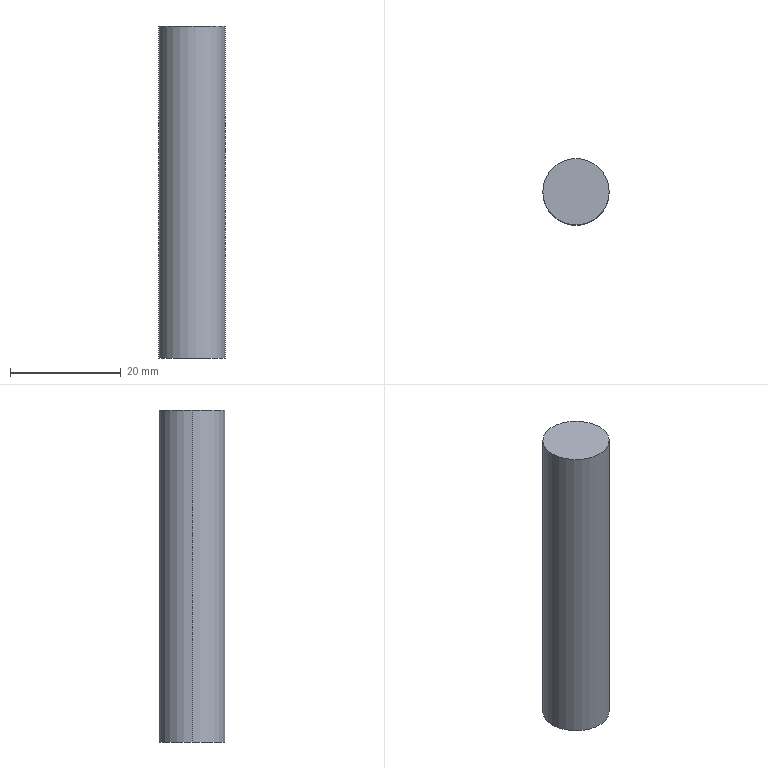Part | SolidWorks | features Extrusion 1 | 1 solid | 4 faces | box 12 x 12 x 60 mm | volume 6786 mm3 | cylinder 2 | plane 2 | commonest cylinder face diameters 12 x2
STEP:
#1=CARTESIAN_POINT('',(6.,0.,-30.));
#2=VERTEX_POINT('',#1);
#3=CARTESIAN_POINT('',(-6.,0.,-30.));
#4=VERTEX_POINT('',#3);
#5=CARTESIAN_POINT('',(0.,0.,-30.));
#6=DIRECTION('',(0.,0.,1.));
#7=DIRECTION('',(1.,0.,0.));
#8=AXIS2_PLACEMENT_3D('',#5,#6,#7);
#9=CIRCLE('',#8,6.);
#10=EDGE_CURVE('',#2,#4,#9,.T.);
#11=ORIENTED_EDGE('',*,*,#10,.T.);
#12=CARTESIAN_POINT('',(-6.,0.,30.));
#13=VERTEX_POINT('',#12);
#14=CARTESIAN_POINT('',(-6.,0.,-30.));
#15=DIRECTION('',(0.,0.,1.));
#16=VECTOR('',#15,1000.);
#17=LINE('',#14,#16);
#18=EDGE_CURVE('',#4,#13,#17,.T.);
#19=ORIENTED_EDGE('',*,*,#18,.T.);
#20=CARTESIAN_POINT('',(6.,0.,30.));
#21=VERTEX_POINT('',#20);
#22=CARTESIAN_POINT('',(0.,0.,30.));
#23=DIRECTION('',(0.,0.,1.));
#24=DIRECTION('',(1.,0.,0.));
#25=AXIS2_PLACEMENT_3D('',#22,#23,#24);
#26=CIRCLE('',#25,6.);
#27=EDGE_CURVE('',#21,#13,#26,.T.);
#28=ORIENTED_EDGE('',*,*,#27,.F.);
#29=CARTESIAN_POINT('',(6.,0.,-30.));
#30=DIRECTION('',(0.,0.,1.));
#31=VECTOR('',#30,1000.);
#32=LINE('',#29,#31);
#33=EDGE_CURVE('',#2,#21,#32,.T.);
#34=ORIENTED_EDGE('',*,*,#33,.F.);
#35=EDGE_LOOP('',(#11,#19,#28,#34));
#36=FACE_OUTER_BOUND('',#35,.T.);
#37=CARTESIAN_POINT('',(0.,0.,-30.));
#38=DIRECTION('',(0.,0.,1.));
#39=DIRECTION('',(1.,0.,0.));
#40=AXIS2_PLACEMENT_3D('',#37,#38,#39);
#41=CYLINDRICAL_SURFACE('',#40,6.);
#42=ADVANCED_FACE('',(#36),#41,.T.);
#43=ORIENTED_EDGE('',*,*,#18,.F.);
#44=CARTESIAN_POINT('',(0.,0.,-30.));
#45=DIRECTION('',(0.,0.,1.));
#46=DIRECTION('',(1.,0.,0.));
#47=AXIS2_PLACEMENT_3D('',#44,#45,#46);
#48=CIRCLE('',#47,6.);
#49=EDGE_CURVE('',#4,#2,#48,.T.);
#50=ORIENTED_EDGE('',*,*,#49,.T.);
#51=ORIENTED_EDGE('',*,*,#33,.T.);
#52=CARTESIAN_POINT('',(0.,0.,30.));
#53=DIRECTION('',(0.,0.,1.));
#54=DIRECTION('',(1.,0.,0.));
#55=AXIS2_PLACEMENT_3D('',#52,#53,#54);
#56=CIRCLE('',#55,6.);
#57=EDGE_CURVE('',#13,#21,#56,.T.);
#58=ORIENTED_EDGE('',*,*,#57,.F.);
#59=EDGE_LOOP('',(#43,#50,#51,#58));
#60=FACE_OUTER_BOUND('',#59,.T.);
#61=CARTESIAN_POINT('',(0.,0.,-30.));
#62=DIRECTION('',(0.,0.,1.));
#63=DIRECTION('',(1.,0.,0.));
#64=AXIS2_PLACEMENT_3D('',#61,#62,#63);
#65=CYLINDRICAL_SURFACE('',#64,6.);
#66=ADVANCED_FACE('',(#60),#65,.T.);
#67=ORIENTED_EDGE('',*,*,#10,.F.);
#68=ORIENTED_EDGE('',*,*,#49,.F.);
#69=EDGE_LOOP('',(#67,#68));
#70=FACE_OUTER_BOUND('',#69,.T.);
#71=CARTESIAN_POINT('',(0.,0.,-30.));
#72=DIRECTION('',(0.,0.,1.));
#73=DIRECTION('',(1.,0.,0.));
#74=AXIS2_PLACEMENT_3D('',#71,#72,#73);
#75=PLANE('',#74);
#76=ADVANCED_FACE('',(#70),#75,.F.);
#77=ORIENTED_EDGE('',*,*,#27,.T.);
#78=ORIENTED_EDGE('',*,*,#57,.T.);
#79=EDGE_LOOP('',(#77,#78));
#80=FACE_OUTER_BOUND('',#79,.T.);
#81=CARTESIAN_POINT('',(0.,0.,30.));
#82=DIRECTION('',(0.,0.,1.));
#83=DIRECTION('',(1.,0.,0.));
#84=AXIS2_PLACEMENT_3D('',#81,#82,#83);
#85=PLANE('',#84);
#86=ADVANCED_FACE('',(#80),#85,.T.);
#87=CLOSED_SHELL('',(#42,#66,#76,#86));
#88=MANIFOLD_SOLID_BREP('',#87);
#89=CARTESIAN_POINT('',(0.,0.,0.));
#90=DIRECTION('',(0.,0.,1.));
#91=DIRECTION('',(1.,0.,0.));
#92=AXIS2_PLACEMENT_3D('',#89,#90,#91);
#93=(LENGTH_UNIT()NAMED_UNIT(*)SI_UNIT(.MILLI.,.METRE.));
#94=UNCERTAINTY_MEASURE_WITH_UNIT(LENGTH_MEASURE(0.00001),#93,'','');
#95=(NAMED_UNIT(*)PLANE_ANGLE_UNIT()SI_UNIT($,.RADIAN.));
#96=(NAMED_UNIT(*)SI_UNIT($,.STERADIAN.)SOLID_ANGLE_UNIT());
#97=(GEOMETRIC_REPRESENTATION_CONTEXT(3)GLOBAL_UNCERTAINTY_ASSIGNED_CONTEXT((#94))GLOBAL_UNIT_ASSIGNED_CONTEXT((#93,#95,#96))REPRESENTATION_CONTEXT('',''));
#98=ADVANCED_BREP_SHAPE_REPRESENTATION('',(#88,#92),#97);